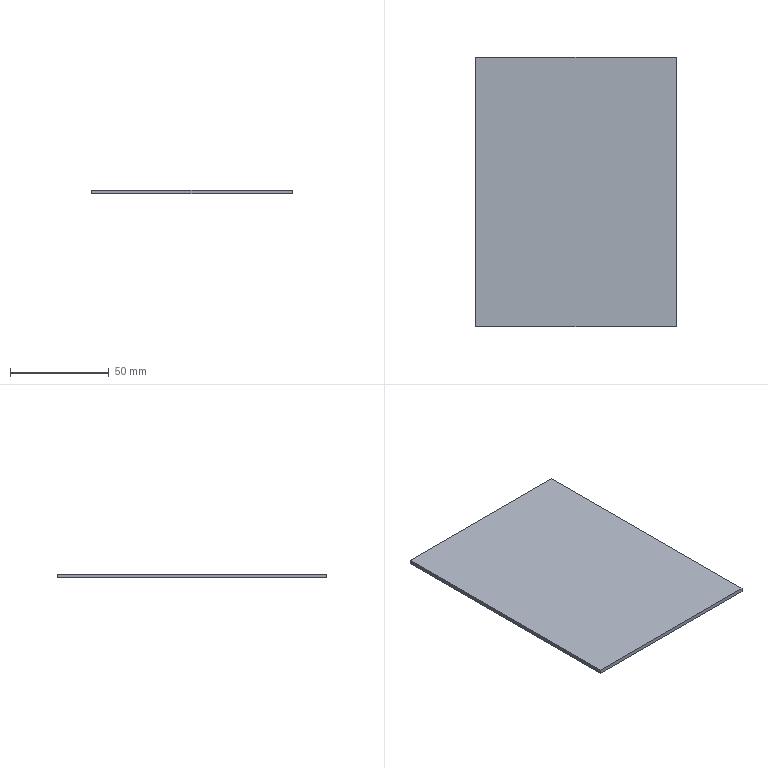Part | SolidWorks | features Extrusion 1 | 1 solid | 6 faces | box 101.6 x 136.525 x 2 mm | volume 27742 mm3 | plane 6
STEP:
#1=CARTESIAN_POINT('',(0.,136.525,0.));
#2=VERTEX_POINT('',#1);
#3=CARTESIAN_POINT('',(0.,0.,0.));
#4=VERTEX_POINT('',#3);
#5=CARTESIAN_POINT('',(0.,0.,0.));
#6=DIRECTION('',(0.,-1.,0.));
#7=VECTOR('',#6,1000.);
#8=LINE('',#5,#7);
#9=EDGE_CURVE('',#2,#4,#8,.T.);
#10=ORIENTED_EDGE('',*,*,#9,.T.);
#11=CARTESIAN_POINT('',(0.,0.,2.));
#12=VERTEX_POINT('',#11);
#13=CARTESIAN_POINT('',(0.,0.,2.));
#14=DIRECTION('',(0.,0.,-1.));
#15=VECTOR('',#14,1000.);
#16=LINE('',#13,#15);
#17=EDGE_CURVE('',#12,#4,#16,.T.);
#18=ORIENTED_EDGE('',*,*,#17,.F.);
#19=CARTESIAN_POINT('',(0.,136.525,2.));
#20=VERTEX_POINT('',#19);
#21=CARTESIAN_POINT('',(0.,0.,2.));
#22=DIRECTION('',(0.,-1.,0.));
#23=VECTOR('',#22,1000.);
#24=LINE('',#21,#23);
#25=EDGE_CURVE('',#20,#12,#24,.T.);
#26=ORIENTED_EDGE('',*,*,#25,.F.);
#27=CARTESIAN_POINT('',(0.,136.525,2.));
#28=DIRECTION('',(0.,0.,-1.));
#29=VECTOR('',#28,1000.);
#30=LINE('',#27,#29);
#31=EDGE_CURVE('',#20,#2,#30,.T.);
#32=ORIENTED_EDGE('',*,*,#31,.T.);
#33=EDGE_LOOP('',(#10,#18,#26,#32));
#34=FACE_OUTER_BOUND('',#33,.T.);
#35=CARTESIAN_POINT('',(0.,0.,2.));
#36=DIRECTION('',(1.,0.,0.));
#37=DIRECTION('',(0.,0.,-1.));
#38=AXIS2_PLACEMENT_3D('',#35,#36,#37);
#39=PLANE('',#38);
#40=ADVANCED_FACE('',(#34),#39,.F.);
#41=CARTESIAN_POINT('',(101.6,0.,0.));
#42=VERTEX_POINT('',#41);
#43=CARTESIAN_POINT('',(0.,0.,0.));
#44=DIRECTION('',(1.,0.,0.));
#45=VECTOR('',#44,1000.);
#46=LINE('',#43,#45);
#47=EDGE_CURVE('',#4,#42,#46,.T.);
#48=ORIENTED_EDGE('',*,*,#47,.T.);
#49=CARTESIAN_POINT('',(101.6,0.,2.));
#50=VERTEX_POINT('',#49);
#51=CARTESIAN_POINT('',(101.6,0.,2.));
#52=DIRECTION('',(0.,0.,-1.));
#53=VECTOR('',#52,1000.);
#54=LINE('',#51,#53);
#55=EDGE_CURVE('',#50,#42,#54,.T.);
#56=ORIENTED_EDGE('',*,*,#55,.F.);
#57=CARTESIAN_POINT('',(0.,0.,2.));
#58=DIRECTION('',(1.,0.,0.));
#59=VECTOR('',#58,1000.);
#60=LINE('',#57,#59);
#61=EDGE_CURVE('',#12,#50,#60,.T.);
#62=ORIENTED_EDGE('',*,*,#61,.F.);
#63=ORIENTED_EDGE('',*,*,#17,.T.);
#64=EDGE_LOOP('',(#48,#56,#62,#63));
#65=FACE_OUTER_BOUND('',#64,.T.);
#66=CARTESIAN_POINT('',(0.,0.,2.));
#67=DIRECTION('',(0.,1.,0.));
#68=DIRECTION('',(0.,0.,1.));
#69=AXIS2_PLACEMENT_3D('',#66,#67,#68);
#70=PLANE('',#69);
#71=ADVANCED_FACE('',(#65),#70,.F.);
#72=CARTESIAN_POINT('',(101.6,136.525,0.));
#73=VERTEX_POINT('',#72);
#74=CARTESIAN_POINT('',(101.6,0.,0.));
#75=DIRECTION('',(0.,1.,0.));
#76=VECTOR('',#75,1000.);
#77=LINE('',#74,#76);
#78=EDGE_CURVE('',#42,#73,#77,.T.);
#79=ORIENTED_EDGE('',*,*,#78,.T.);
#80=CARTESIAN_POINT('',(101.6,136.525,2.));
#81=VERTEX_POINT('',#80);
#82=CARTESIAN_POINT('',(101.6,136.525,2.));
#83=DIRECTION('',(0.,0.,-1.));
#84=VECTOR('',#83,1000.);
#85=LINE('',#82,#84);
#86=EDGE_CURVE('',#81,#73,#85,.T.);
#87=ORIENTED_EDGE('',*,*,#86,.F.);
#88=CARTESIAN_POINT('',(101.6,0.,2.));
#89=DIRECTION('',(0.,1.,0.));
#90=VECTOR('',#89,1000.);
#91=LINE('',#88,#90);
#92=EDGE_CURVE('',#50,#81,#91,.T.);
#93=ORIENTED_EDGE('',*,*,#92,.F.);
#94=ORIENTED_EDGE('',*,*,#55,.T.);
#95=EDGE_LOOP('',(#79,#87,#93,#94));
#96=FACE_OUTER_BOUND('',#95,.T.);
#97=CARTESIAN_POINT('',(101.6,0.,2.));
#98=DIRECTION('',(-1.,0.,0.));
#99=DIRECTION('',(0.,0.,1.));
#100=AXIS2_PLACEMENT_3D('',#97,#98,#99);
#101=PLANE('',#100);
#102=ADVANCED_FACE('',(#96),#101,.F.);
#103=CARTESIAN_POINT('',(0.,136.525,0.));
#104=DIRECTION('',(-1.,0.,0.));
#105=VECTOR('',#104,1000.);
#106=LINE('',#103,#105);
#107=EDGE_CURVE('',#73,#2,#106,.T.);
#108=ORIENTED_EDGE('',*,*,#107,.T.);
#109=ORIENTED_EDGE('',*,*,#31,.F.);
#110=CARTESIAN_POINT('',(0.,136.525,2.));
#111=DIRECTION('',(-1.,0.,0.));
#112=VECTOR('',#111,1000.);
#113=LINE('',#110,#112);
#114=EDGE_CURVE('',#81,#20,#113,.T.);
#115=ORIENTED_EDGE('',*,*,#114,.F.);
#116=ORIENTED_EDGE('',*,*,#86,.T.);
#117=EDGE_LOOP('',(#108,#109,#115,#116));
#118=FACE_OUTER_BOUND('',#117,.T.);
#119=CARTESIAN_POINT('',(0.,136.525,2.));
#120=DIRECTION('',(0.,-1.,0.));
#121=DIRECTION('',(0.,0.,-1.));
#122=AXIS2_PLACEMENT_3D('',#119,#120,#121);
#123=PLANE('',#122);
#124=ADVANCED_FACE('',(#118),#123,.F.);
#125=ORIENTED_EDGE('',*,*,#25,.T.);
#126=ORIENTED_EDGE('',*,*,#61,.T.);
#127=ORIENTED_EDGE('',*,*,#92,.T.);
#128=ORIENTED_EDGE('',*,*,#114,.T.);
#129=EDGE_LOOP('',(#125,#126,#127,#128));
#130=FACE_OUTER_BOUND('',#129,.T.);
#131=CARTESIAN_POINT('',(0.,0.,2.));
#132=DIRECTION('',(0.,0.,-1.));
#133=DIRECTION('',(-1.,0.,0.));
#134=AXIS2_PLACEMENT_3D('',#131,#132,#133);
#135=PLANE('',#134);
#136=ADVANCED_FACE('',(#130),#135,.F.);
#137=ORIENTED_EDGE('',*,*,#9,.F.);
#138=ORIENTED_EDGE('',*,*,#107,.F.);
#139=ORIENTED_EDGE('',*,*,#78,.F.);
#140=ORIENTED_EDGE('',*,*,#47,.F.);
#141=EDGE_LOOP('',(#137,#138,#139,#140));
#142=FACE_OUTER_BOUND('',#141,.T.);
#143=CARTESIAN_POINT('',(0.,0.,0.));
#144=DIRECTION('',(0.,0.,-1.));
#145=DIRECTION('',(-1.,0.,0.));
#146=AXIS2_PLACEMENT_3D('',#143,#144,#145);
#147=PLANE('',#146);
#148=ADVANCED_FACE('',(#142),#147,.T.);
#149=CLOSED_SHELL('',(#40,#71,#102,#124,#136,#148));
#150=MANIFOLD_SOLID_BREP('',#149);
#151=CARTESIAN_POINT('',(0.,0.,0.));
#152=DIRECTION('',(0.,0.,1.));
#153=DIRECTION('',(1.,0.,0.));
#154=AXIS2_PLACEMENT_3D('',#151,#152,#153);
#155=(LENGTH_UNIT()NAMED_UNIT(*)SI_UNIT(.MILLI.,.METRE.));
#156=UNCERTAINTY_MEASURE_WITH_UNIT(LENGTH_MEASURE(0.00001),#155,'','');
#157=(NAMED_UNIT(*)PLANE_ANGLE_UNIT()SI_UNIT($,.RADIAN.));
#158=(NAMED_UNIT(*)SI_UNIT($,.STERADIAN.)SOLID_ANGLE_UNIT());
#159=(GEOMETRIC_REPRESENTATION_CONTEXT(3)GLOBAL_UNCERTAINTY_ASSIGNED_CONTEXT((#156))GLOBAL_UNIT_ASSIGNED_CONTEXT((#155,#157,#158))REPRESENTATION_CONTEXT('',''));
#160=ADVANCED_BREP_SHAPE_REPRESENTATION('',(#150,#154),#159);